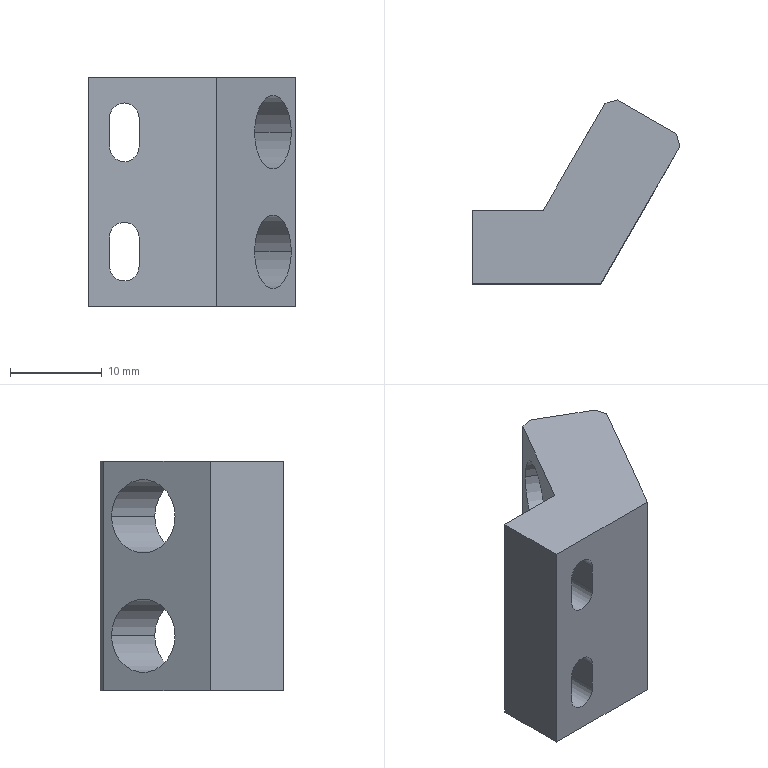Part | SolidWorks | features ICE 15, MoveFace 2, Chamfer 1, Extrusion 1 | 1 solid | 36 faces | box 22.618 x 20.004 x 25 mm | volume 4524 mm3 | plane 20 | cylinder 16 | commonest cylinder face diameters 3.2 x6 6 x6 8 x4
STEP:
#1=CARTESIAN_POINT('',(10.821,-32.,23.6));
#2=VERTEX_POINT('',#1);
#3=CARTESIAN_POINT('',(13.821,-32.,20.6));
#4=VERTEX_POINT('',#3);
#5=CARTESIAN_POINT('',(10.821,-32.,20.6));
#6=DIRECTION('',(0.,1.,0.));
#7=DIRECTION('',(0.,0.,1.));
#8=AXIS2_PLACEMENT_3D('',#5,#6,#7);
#9=CIRCLE('',#8,3.);
#10=EDGE_CURVE('',#2,#4,#9,.T.);
#11=ORIENTED_EDGE('',*,*,#10,.F.);
#12=CARTESIAN_POINT('',(10.821,-28.,23.6));
#13=VERTEX_POINT('',#12);
#14=CARTESIAN_POINT('',(10.821,-32.,23.6));
#15=DIRECTION('',(0.,1.,0.));
#16=VECTOR('',#15,1000.);
#17=LINE('',#14,#16);
#18=EDGE_CURVE('',#2,#13,#17,.T.);
#19=ORIENTED_EDGE('',*,*,#18,.T.);
#20=CARTESIAN_POINT('',(13.821,-28.,20.6));
#21=VERTEX_POINT('',#20);
#22=CARTESIAN_POINT('',(10.821,-28.,20.6));
#23=DIRECTION('',(0.,1.,0.));
#24=DIRECTION('',(0.,0.,1.));
#25=AXIS2_PLACEMENT_3D('',#22,#23,#24);
#26=CIRCLE('',#25,3.);
#27=EDGE_CURVE('',#13,#21,#26,.T.);
#28=ORIENTED_EDGE('',*,*,#27,.T.);
#29=CARTESIAN_POINT('',(13.821,-32.,20.6));
#30=DIRECTION('',(0.,1.,0.));
#31=VECTOR('',#30,1000.);
#32=LINE('',#29,#31);
#33=EDGE_CURVE('',#4,#21,#32,.T.);
#34=ORIENTED_EDGE('',*,*,#33,.F.);
#35=EDGE_LOOP('',(#11,#19,#28,#34));
#36=FACE_OUTER_BOUND('',#35,.T.);
#37=CARTESIAN_POINT('',(10.821,-32.,20.6));
#38=DIRECTION('',(0.,1.,0.));
#39=DIRECTION('',(0.,0.,1.));
#40=AXIS2_PLACEMENT_3D('',#37,#38,#39);
#41=CYLINDRICAL_SURFACE('',#40,3.);
#42=ADVANCED_FACE('',(#36),#41,.F.);
#43=CARTESIAN_POINT('',(10.821,-32.,10.6));
#44=VERTEX_POINT('',#43);
#45=CARTESIAN_POINT('',(13.821,-32.,7.6));
#46=VERTEX_POINT('',#45);
#47=CARTESIAN_POINT('',(10.821,-32.,7.6));
#48=DIRECTION('',(0.,1.,0.));
#49=DIRECTION('',(0.,0.,1.));
#50=AXIS2_PLACEMENT_3D('',#47,#48,#49);
#51=CIRCLE('',#50,3.);
#52=EDGE_CURVE('',#44,#46,#51,.T.);
#53=ORIENTED_EDGE('',*,*,#52,.F.);
#54=CARTESIAN_POINT('',(10.821,-28.,10.6));
#55=VERTEX_POINT('',#54);
#56=CARTESIAN_POINT('',(10.821,-32.,10.6));
#57=DIRECTION('',(0.,1.,0.));
#58=VECTOR('',#57,1000.);
#59=LINE('',#56,#58);
#60=EDGE_CURVE('',#44,#55,#59,.T.);
#61=ORIENTED_EDGE('',*,*,#60,.T.);
#62=CARTESIAN_POINT('',(13.821,-28.,7.6));
#63=VERTEX_POINT('',#62);
#64=CARTESIAN_POINT('',(10.821,-28.,7.6));
#65=DIRECTION('',(0.,1.,0.));
#66=DIRECTION('',(0.,0.,1.));
#67=AXIS2_PLACEMENT_3D('',#64,#65,#66);
#68=CIRCLE('',#67,3.);
#69=EDGE_CURVE('',#55,#63,#68,.T.);
#70=ORIENTED_EDGE('',*,*,#69,.T.);
#71=CARTESIAN_POINT('',(13.821,-32.,7.6));
#72=DIRECTION('',(0.,1.,0.));
#73=VECTOR('',#72,1000.);
#74=LINE('',#71,#73);
#75=EDGE_CURVE('',#46,#63,#74,.T.);
#76=ORIENTED_EDGE('',*,*,#75,.F.);
#77=EDGE_LOOP('',(#53,#61,#70,#76));
#78=FACE_OUTER_BOUND('',#77,.T.);
#79=CARTESIAN_POINT('',(10.821,-32.,7.6));
#80=DIRECTION('',(0.,1.,0.));
#81=DIRECTION('',(0.,0.,1.));
#82=AXIS2_PLACEMENT_3D('',#79,#80,#81);
#83=CYLINDRICAL_SURFACE('',#82,3.);
#84=ADVANCED_FACE('',(#78),#83,.F.);
#85=CARTESIAN_POINT('',(25.,-28.868,6.));
#86=VERTEX_POINT('',#85);
#87=CARTESIAN_POINT('',(29.,-21.939,6.));
#88=VERTEX_POINT('',#87);
#89=CARTESIAN_POINT('',(27.,-25.403,6.));
#90=DIRECTION('',(0.866,-0.5,0.));
#91=DIRECTION('',(-0.5,-0.866,0.));
#92=AXIS2_PLACEMENT_3D('',#89,#90,#91);
#93=CIRCLE('',#92,4.);
#94=EDGE_CURVE('',#86,#88,#93,.T.);
#95=ORIENTED_EDGE('',*,*,#94,.T.);
#96=CARTESIAN_POINT('',(20.84,-17.228,6.));
#97=VERTEX_POINT('',#96);
#98=CARTESIAN_POINT('',(52.301,-35.392,6.));
#99=DIRECTION('',(-0.866,0.5,0.));
#100=VECTOR('',#99,1000.);
#101=LINE('',#98,#100);
#102=EDGE_CURVE('',#88,#97,#101,.T.);
#103=ORIENTED_EDGE('',*,*,#102,.T.);
#104=CARTESIAN_POINT('',(16.84,-24.156,6.));
#105=VERTEX_POINT('',#104);
#106=CARTESIAN_POINT('',(18.84,-20.692,6.));
#107=DIRECTION('',(-0.866,0.5,0.));
#108=DIRECTION('',(0.5,0.866,0.));
#109=AXIS2_PLACEMENT_3D('',#106,#107,#108);
#110=CIRCLE('',#109,4.);
#111=EDGE_CURVE('',#97,#105,#110,.T.);
#112=ORIENTED_EDGE('',*,*,#111,.T.);
#113=CARTESIAN_POINT('',(48.301,-42.321,6.));
#114=DIRECTION('',(-0.866,0.5,0.));
#115=VECTOR('',#114,1000.);
#116=LINE('',#113,#115);
#117=EDGE_CURVE('',#86,#105,#116,.T.);
#118=ORIENTED_EDGE('',*,*,#117,.F.);
#119=EDGE_LOOP('',(#95,#103,#112,#118));
#120=FACE_OUTER_BOUND('',#119,.T.);
#121=CARTESIAN_POINT('',(50.301,-38.856,6.));
#122=DIRECTION('',(-0.866,0.5,0.));
#123=DIRECTION('',(-0.5,-0.866,0.));
#124=AXIS2_PLACEMENT_3D('',#121,#122,#123);
#125=CYLINDRICAL_SURFACE('',#124,4.);
#126=ADVANCED_FACE('',(#120),#125,.F.);
#127=CARTESIAN_POINT('',(25.,-28.868,19.));
#128=VERTEX_POINT('',#127);
#129=CARTESIAN_POINT('',(29.,-21.939,19.));
#130=VERTEX_POINT('',#129);
#131=CARTESIAN_POINT('',(27.,-25.403,19.));
#132=DIRECTION('',(0.866,-0.5,0.));
#133=DIRECTION('',(-0.5,-0.866,0.));
#134=AXIS2_PLACEMENT_3D('',#131,#132,#133);
#135=CIRCLE('',#134,4.);
#136=EDGE_CURVE('',#128,#130,#135,.T.);
#137=ORIENTED_EDGE('',*,*,#136,.T.);
#138=CARTESIAN_POINT('',(20.84,-17.228,19.));
#139=VERTEX_POINT('',#138);
#140=CARTESIAN_POINT('',(52.301,-35.392,19.));
#141=DIRECTION('',(-0.866,0.5,0.));
#142=VECTOR('',#141,1000.);
#143=LINE('',#140,#142);
#144=EDGE_CURVE('',#130,#139,#143,.T.);
#145=ORIENTED_EDGE('',*,*,#144,.T.);
#146=CARTESIAN_POINT('',(16.84,-24.156,19.));
#147=VERTEX_POINT('',#146);
#148=CARTESIAN_POINT('',(18.84,-20.692,19.));
#149=DIRECTION('',(-0.866,0.5,0.));
#150=DIRECTION('',(0.5,0.866,0.));
#151=AXIS2_PLACEMENT_3D('',#148,#149,#150);
#152=CIRCLE('',#151,4.);
#153=EDGE_CURVE('',#139,#147,#152,.T.);
#154=ORIENTED_EDGE('',*,*,#153,.T.);
#155=CARTESIAN_POINT('',(48.301,-42.321,19.));
#156=DIRECTION('',(-0.866,0.5,0.));
#157=VECTOR('',#156,1000.);
#158=LINE('',#155,#157);
#159=EDGE_CURVE('',#128,#147,#158,.T.);
#160=ORIENTED_EDGE('',*,*,#159,.F.);
#161=EDGE_LOOP('',(#137,#145,#154,#160));
#162=FACE_OUTER_BOUND('',#161,.T.);
#163=CARTESIAN_POINT('',(50.301,-38.856,19.));
#164=DIRECTION('',(-0.866,0.5,0.));
#165=DIRECTION('',(-0.5,-0.866,0.));
#166=AXIS2_PLACEMENT_3D('',#163,#164,#165);
#167=CYLINDRICAL_SURFACE('',#166,4.);
#168=ADVANCED_FACE('',(#162),#167,.F.);
#169=CARTESIAN_POINT('',(10.821,-36.,9.2));
#170=VERTEX_POINT('',#169);
#171=CARTESIAN_POINT('',(12.421,-36.,7.6));
#172=VERTEX_POINT('',#171);
#173=CARTESIAN_POINT('',(10.821,-36.,7.6));
#174=DIRECTION('',(0.,1.,0.));
#175=DIRECTION('',(0.,0.,1.));
#176=AXIS2_PLACEMENT_3D('',#173,#174,#175);
#177=CIRCLE('',#176,1.6);
#178=EDGE_CURVE('',#170,#172,#177,.T.);
#179=ORIENTED_EDGE('',*,*,#178,.F.);
#180=CARTESIAN_POINT('',(10.821,-32.,9.2));
#181=VERTEX_POINT('',#180);
#182=CARTESIAN_POINT('',(10.821,-38.,9.2));
#183=DIRECTION('',(0.,1.,0.));
#184=VECTOR('',#183,1000.);
#185=LINE('',#182,#184);
#186=EDGE_CURVE('',#170,#181,#185,.T.);
#187=ORIENTED_EDGE('',*,*,#186,.T.);
#188=CARTESIAN_POINT('',(12.421,-32.,7.6));
#189=VERTEX_POINT('',#188);
#190=CARTESIAN_POINT('',(10.821,-32.,7.6));
#191=DIRECTION('',(0.,-1.,0.));
#192=DIRECTION('',(0.,0.,1.));
#193=AXIS2_PLACEMENT_3D('',#190,#191,#192);
#194=CIRCLE('',#193,1.6);
#195=EDGE_CURVE('',#189,#181,#194,.T.);
#196=ORIENTED_EDGE('',*,*,#195,.F.);
#197=CARTESIAN_POINT('',(12.421,-38.,7.6));
#198=DIRECTION('',(0.,1.,0.));
#199=VECTOR('',#198,1000.);
#200=LINE('',#197,#199);
#201=EDGE_CURVE('',#172,#189,#200,.T.);
#202=ORIENTED_EDGE('',*,*,#201,.F.);
#203=EDGE_LOOP('',(#179,#187,#196,#202));
#204=FACE_OUTER_BOUND('',#203,.T.);
#205=CARTESIAN_POINT('',(10.821,-38.,7.6));
#206=DIRECTION('',(0.,1.,0.));
#207=DIRECTION('',(0.,0.,1.));
#208=AXIS2_PLACEMENT_3D('',#205,#206,#207);
#209=CYLINDRICAL_SURFACE('',#208,1.6);
#210=ADVANCED_FACE('',(#204),#209,.F.);
#211=CARTESIAN_POINT('',(10.821,-36.,22.2));
#212=VERTEX_POINT('',#211);
#213=CARTESIAN_POINT('',(12.421,-36.,20.6));
#214=VERTEX_POINT('',#213);
#215=CARTESIAN_POINT('',(10.821,-36.,20.6));
#216=DIRECTION('',(0.,1.,0.));
#217=DIRECTION('',(0.,0.,1.));
#218=AXIS2_PLACEMENT_3D('',#215,#216,#217);
#219=CIRCLE('',#218,1.6);
#220=EDGE_CURVE('',#212,#214,#219,.T.);
#221=ORIENTED_EDGE('',*,*,#220,.F.);
#222=CARTESIAN_POINT('',(10.821,-32.,22.2));
#223=VERTEX_POINT('',#222);
#224=CARTESIAN_POINT('',(10.821,-38.,22.2));
#225=DIRECTION('',(0.,1.,0.));
#226=VECTOR('',#225,1000.);
#227=LINE('',#224,#226);
#228=EDGE_CURVE('',#212,#223,#227,.T.);
#229=ORIENTED_EDGE('',*,*,#228,.T.);
#230=CARTESIAN_POINT('',(12.421,-32.,20.6));
#231=VERTEX_POINT('',#230);
#232=CARTESIAN_POINT('',(10.821,-32.,20.6));
#233=DIRECTION('',(0.,-1.,0.));
#234=DIRECTION('',(0.,0.,1.));
#235=AXIS2_PLACEMENT_3D('',#232,#233,#234);
#236=CIRCLE('',#235,1.6);
#237=EDGE_CURVE('',#231,#223,#236,.T.);
#238=ORIENTED_EDGE('',*,*,#237,.F.);
#239=CARTESIAN_POINT('',(12.421,-38.,20.6));
#240=DIRECTION('',(0.,1.,0.));
#241=VECTOR('',#240,1000.);
#242=LINE('',#239,#241);
#243=EDGE_CURVE('',#214,#231,#242,.T.);
#244=ORIENTED_EDGE('',*,*,#243,.F.);
#245=EDGE_LOOP('',(#221,#229,#238,#244));
#246=FACE_OUTER_BOUND('',#245,.T.);
#247=CARTESIAN_POINT('',(10.821,-38.,20.6));
#248=DIRECTION('',(0.,1.,0.));
#249=DIRECTION('',(0.,0.,1.));
#250=AXIS2_PLACEMENT_3D('',#247,#248,#249);
#251=CYLINDRICAL_SURFACE('',#250,1.6);
#252=ADVANCED_FACE('',(#246),#251,.F.);
#253=CARTESIAN_POINT('',(9.221,-32.,17.4));
#254=VERTEX_POINT('',#253);
#255=CARTESIAN_POINT('',(12.421,-32.,17.4));
#256=VERTEX_POINT('',#255);
#257=CARTESIAN_POINT('',(10.821,-32.,17.4));
#258=DIRECTION('',(0.,-1.,0.));
#259=DIRECTION('',(0.,0.,1.));
#260=AXIS2_PLACEMENT_3D('',#257,#258,#259);
#261=CIRCLE('',#260,1.6);
#262=EDGE_CURVE('',#254,#256,#261,.T.);
#263=ORIENTED_EDGE('',*,*,#262,.F.);
#264=CARTESIAN_POINT('',(9.221,-36.,17.4));
#265=VERTEX_POINT('',#264);
#266=CARTESIAN_POINT('',(9.221,-38.,17.4));
#267=DIRECTION('',(0.,1.,0.));
#268=VECTOR('',#267,1000.);
#269=LINE('',#266,#268);
#270=EDGE_CURVE('',#265,#254,#269,.T.);
#271=ORIENTED_EDGE('',*,*,#270,.F.);
#272=CARTESIAN_POINT('',(12.421,-36.,17.4));
#273=VERTEX_POINT('',#272);
#274=CARTESIAN_POINT('',(10.821,-36.,17.4));
#275=DIRECTION('',(0.,1.,0.));
#276=DIRECTION('',(0.,0.,1.));
#277=AXIS2_PLACEMENT_3D('',#274,#275,#276);
#278=CIRCLE('',#277,1.6);
#279=EDGE_CURVE('',#273,#265,#278,.T.);
#280=ORIENTED_EDGE('',*,*,#279,.F.);
#281=CARTESIAN_POINT('',(12.421,-38.,17.4));
#282=DIRECTION('',(0.,1.,0.));
#283=VECTOR('',#282,1000.);
#284=LINE('',#281,#283);
#285=EDGE_CURVE('',#273,#256,#284,.T.);
#286=ORIENTED_EDGE('',*,*,#285,.T.);
#287=EDGE_LOOP('',(#263,#271,#280,#286));
#288=FACE_OUTER_BOUND('',#287,.T.);
#289=CARTESIAN_POINT('',(10.821,-38.,17.4));
#290=DIRECTION('',(0.,1.,0.));
#291=DIRECTION('',(0.,0.,1.));
#292=AXIS2_PLACEMENT_3D('',#289,#290,#291);
#293=CYLINDRICAL_SURFACE('',#292,1.6);
#294=ADVANCED_FACE('',(#288),#293,.F.);
#295=ORIENTED_EDGE('',*,*,#228,.F.);
#296=CARTESIAN_POINT('',(9.221,-36.,20.6));
#297=VERTEX_POINT('',#296);
#298=CARTESIAN_POINT('',(10.821,-36.,20.6));
#299=DIRECTION('',(0.,1.,0.));
#300=DIRECTION('',(0.,0.,1.));
#301=AXIS2_PLACEMENT_3D('',#298,#299,#300);
#302=CIRCLE('',#301,1.6);
#303=EDGE_CURVE('',#297,#212,#302,.T.);
#304=ORIENTED_EDGE('',*,*,#303,.F.);
#305=CARTESIAN_POINT('',(9.221,-32.,20.6));
#306=VERTEX_POINT('',#305);
#307=CARTESIAN_POINT('',(9.221,-38.,20.6));
#308=DIRECTION('',(0.,1.,0.));
#309=VECTOR('',#308,1000.);
#310=LINE('',#307,#309);
#311=EDGE_CURVE('',#297,#306,#310,.T.);
#312=ORIENTED_EDGE('',*,*,#311,.T.);
#313=CARTESIAN_POINT('',(10.821,-32.,20.6));
#314=DIRECTION('',(0.,-1.,0.));
#315=DIRECTION('',(0.,0.,1.));
#316=AXIS2_PLACEMENT_3D('',#313,#314,#315);
#317=CIRCLE('',#316,1.6);
#318=EDGE_CURVE('',#223,#306,#317,.T.);
#319=ORIENTED_EDGE('',*,*,#318,.F.);
#320=EDGE_LOOP('',(#295,#304,#312,#319));
#321=FACE_OUTER_BOUND('',#320,.T.);
#322=CARTESIAN_POINT('',(10.821,-38.,20.6));
#323=DIRECTION('',(0.,1.,0.));
#324=DIRECTION('',(0.,0.,1.));
#325=AXIS2_PLACEMENT_3D('',#322,#323,#324);
#326=CYLINDRICAL_SURFACE('',#325,1.6);
#327=ADVANCED_FACE('',(#321),#326,.F.);
#328=CARTESIAN_POINT('',(12.421,-32.,17.4));
#329=DIRECTION('',(0.,0.,1.));
#330=VECTOR('',#329,1000.);
#331=LINE('',#328,#330);
#332=EDGE_CURVE('',#256,#231,#331,.T.);
#333=ORIENTED_EDGE('',*,*,#332,.F.);
#334=ORIENTED_EDGE('',*,*,#285,.F.);
#335=CARTESIAN_POINT('',(12.421,-36.,-6.));
#336=DIRECTION('',(0.,0.,-1.));
#337=VECTOR('',#336,1000.);
#338=LINE('',#335,#337);
#339=EDGE_CURVE('',#214,#273,#338,.T.);
#340=ORIENTED_EDGE('',*,*,#339,.F.);
#341=ORIENTED_EDGE('',*,*,#243,.T.);
#342=EDGE_LOOP('',(#333,#334,#340,#341));
#343=FACE_OUTER_BOUND('',#342,.T.);
#344=CARTESIAN_POINT('',(12.421,-38.,17.4));
#345=DIRECTION('',(1.,0.,0.));
#346=DIRECTION('',(0.,0.,-1.));
#347=AXIS2_PLACEMENT_3D('',#344,#345,#346);
#348=PLANE('',#347);
#349=ADVANCED_FACE('',(#343),#348,.F.);
#350=CARTESIAN_POINT('',(9.221,-32.,17.4));
#351=DIRECTION('',(0.,0.,-1.));
#352=VECTOR('',#351,1000.);
#353=LINE('',#350,#352);
#354=EDGE_CURVE('',#306,#254,#353,.T.);
#355=ORIENTED_EDGE('',*,*,#354,.F.);
#356=ORIENTED_EDGE('',*,*,#311,.F.);
#357=CARTESIAN_POINT('',(9.221,-36.,-6.));
#358=DIRECTION('',(0.,0.,1.));
#359=VECTOR('',#358,1000.);
#360=LINE('',#357,#359);
#361=EDGE_CURVE('',#265,#297,#360,.T.);
#362=ORIENTED_EDGE('',*,*,#361,.F.);
#363=ORIENTED_EDGE('',*,*,#270,.T.);
#364=EDGE_LOOP('',(#355,#356,#362,#363));
#365=FACE_OUTER_BOUND('',#364,.T.);
#366=CARTESIAN_POINT('',(9.221,-38.,17.4));
#367=DIRECTION('',(-1.,0.,0.));
#368=DIRECTION('',(0.,0.,1.));
#369=AXIS2_PLACEMENT_3D('',#366,#367,#368);
#370=PLANE('',#369);
#371=ADVANCED_FACE('',(#365),#370,.F.);
#372=CARTESIAN_POINT('',(9.221,-32.,4.4));
#373=VERTEX_POINT('',#372);
#374=CARTESIAN_POINT('',(12.421,-32.,4.4));
#375=VERTEX_POINT('',#374);
#376=CARTESIAN_POINT('',(10.821,-32.,4.4));
#377=DIRECTION('',(0.,-1.,0.));
#378=DIRECTION('',(0.,0.,1.));
#379=AXIS2_PLACEMENT_3D('',#376,#377,#378);
#380=CIRCLE('',#379,1.6);
#381=EDGE_CURVE('',#373,#375,#380,.T.);
#382=ORIENTED_EDGE('',*,*,#381,.F.);
#383=CARTESIAN_POINT('',(9.221,-36.,4.4));
#384=VERTEX_POINT('',#383);
#385=CARTESIAN_POINT('',(9.221,-38.,4.4));
#386=DIRECTION('',(0.,1.,0.));
#387=VECTOR('',#386,1000.);
#388=LINE('',#385,#387);
#389=EDGE_CURVE('',#384,#373,#388,.T.);
#390=ORIENTED_EDGE('',*,*,#389,.F.);
#391=CARTESIAN_POINT('',(12.421,-36.,4.4));
#392=VERTEX_POINT('',#391);
#393=CARTESIAN_POINT('',(10.821,-36.,4.4));
#394=DIRECTION('',(0.,1.,0.));
#395=DIRECTION('',(0.,0.,1.));
#396=AXIS2_PLACEMENT_3D('',#393,#394,#395);
#397=CIRCLE('',#396,1.6);
#398=EDGE_CURVE('',#392,#384,#397,.T.);
#399=ORIENTED_EDGE('',*,*,#398,.F.);
#400=CARTESIAN_POINT('',(12.421,-38.,4.4));
#401=DIRECTION('',(0.,1.,0.));
#402=VECTOR('',#401,1000.);
#403=LINE('',#400,#402);
#404=EDGE_CURVE('',#392,#375,#403,.T.);
#405=ORIENTED_EDGE('',*,*,#404,.T.);
#406=EDGE_LOOP('',(#382,#390,#399,#405));
#407=FACE_OUTER_BOUND('',#406,.T.);
#408=CARTESIAN_POINT('',(10.821,-38.,4.4));
#409=DIRECTION('',(0.,1.,0.));
#410=DIRECTION('',(0.,0.,1.));
#411=AXIS2_PLACEMENT_3D('',#408,#409,#410);
#412=CYLINDRICAL_SURFACE('',#411,1.6);
#413=ADVANCED_FACE('',(#407),#412,.F.);
#414=ORIENTED_EDGE('',*,*,#186,.F.);
#415=CARTESIAN_POINT('',(9.221,-36.,7.6));
#416=VERTEX_POINT('',#415);
#417=CARTESIAN_POINT('',(10.821,-36.,7.6));
#418=DIRECTION('',(0.,1.,0.));
#419=DIRECTION('',(0.,0.,1.));
#420=AXIS2_PLACEMENT_3D('',#417,#418,#419);
#421=CIRCLE('',#420,1.6);
#422=EDGE_CURVE('',#416,#170,#421,.T.);
#423=ORIENTED_EDGE('',*,*,#422,.F.);
#424=CARTESIAN_POINT('',(9.221,-32.,7.6));
#425=VERTEX_POINT('',#424);
#426=CARTESIAN_POINT('',(9.221,-38.,7.6));
#427=DIRECTION('',(0.,1.,0.));
#428=VECTOR('',#427,1000.);
#429=LINE('',#426,#428);
#430=EDGE_CURVE('',#416,#425,#429,.T.);
#431=ORIENTED_EDGE('',*,*,#430,.T.);
#432=CARTESIAN_POINT('',(10.821,-32.,7.6));
#433=DIRECTION('',(0.,-1.,0.));
#434=DIRECTION('',(0.,0.,1.));
#435=AXIS2_PLACEMENT_3D('',#432,#433,#434);
#436=CIRCLE('',#435,1.6);
#437=EDGE_CURVE('',#181,#425,#436,.T.);
#438=ORIENTED_EDGE('',*,*,#437,.F.);
#439=EDGE_LOOP('',(#414,#423,#431,#438));
#440=FACE_OUTER_BOUND('',#439,.T.);
#441=CARTESIAN_POINT('',(10.821,-38.,7.6));
#442=DIRECTION('',(0.,1.,0.));
#443=DIRECTION('',(0.,0.,1.));
#444=AXIS2_PLACEMENT_3D('',#441,#442,#443);
#445=CYLINDRICAL_SURFACE('',#444,1.6);
#446=ADVANCED_FACE('',(#440),#445,.F.);
#447=CARTESIAN_POINT('',(12.421,-32.,4.4));
#448=DIRECTION('',(0.,0.,1.));
#449=VECTOR('',#448,1000.);
#450=LINE('',#447,#449);
#451=EDGE_CURVE('',#375,#189,#450,.T.);
#452=ORIENTED_EDGE('',*,*,#451,.F.);
#453=ORIENTED_EDGE('',*,*,#404,.F.);
#454=CARTESIAN_POINT('',(12.421,-36.,-6.));
#455=DIRECTION('',(0.,0.,-1.));
#456=VECTOR('',#455,1000.);
#457=LINE('',#454,#456);
#458=EDGE_CURVE('',#172,#392,#457,.T.);
#459=ORIENTED_EDGE('',*,*,#458,.F.);
#460=ORIENTED_EDGE('',*,*,#201,.T.);
#461=EDGE_LOOP('',(#452,#453,#459,#460));
#462=FACE_OUTER_BOUND('',#461,.T.);
#463=CARTESIAN_POINT('',(12.421,-38.,4.4));
#464=DIRECTION('',(1.,0.,0.));
#465=DIRECTION('',(0.,0.,-1.));
#466=AXIS2_PLACEMENT_3D('',#463,#464,#465);
#467=PLANE('',#466);
#468=ADVANCED_FACE('',(#462),#467,.F.);
#469=CARTESIAN_POINT('',(9.221,-32.,4.4));
#470=DIRECTION('',(0.,0.,-1.));
#471=VECTOR('',#470,1000.);
#472=LINE('',#469,#471);
#473=EDGE_CURVE('',#425,#373,#472,.T.);
#474=ORIENTED_EDGE('',*,*,#473,.F.);
#475=ORIENTED_EDGE('',*,*,#430,.F.);
#476=CARTESIAN_POINT('',(9.221,-36.,-6.));
#477=DIRECTION('',(0.,0.,1.));
#478=VECTOR('',#477,1000.);
#479=LINE('',#476,#478);
#480=EDGE_CURVE('',#384,#416,#479,.T.);
#481=ORIENTED_EDGE('',*,*,#480,.F.);
#482=ORIENTED_EDGE('',*,*,#389,.T.);
#483=EDGE_LOOP('',(#474,#475,#481,#482));
#484=FACE_OUTER_BOUND('',#483,.T.);
#485=CARTESIAN_POINT('',(9.221,-38.,4.4));
#486=DIRECTION('',(-1.,0.,0.));
#487=DIRECTION('',(0.,0.,1.));
#488=AXIS2_PLACEMENT_3D('',#485,#486,#487);
#489=PLANE('',#488);
#490=ADVANCED_FACE('',(#484),#489,.F.);
#491=CARTESIAN_POINT('',(18.84,-20.692,19.));
#492=DIRECTION('',(-0.866,0.5,0.));
#493=DIRECTION('',(0.5,0.866,0.));
#494=AXIS2_PLACEMENT_3D('',#491,#492,#493);
#495=CIRCLE('',#494,4.);
#496=EDGE_CURVE('',#147,#139,#495,.T.);
#497=ORIENTED_EDGE('',*,*,#496,.F.);
#498=ORIENTED_EDGE('',*,*,#153,.F.);
#499=EDGE_LOOP('',(#497,#498));
#500=FACE_BOUND('',#499,.T.);
#501=CARTESIAN_POINT('',(18.84,-20.692,6.));
#502=DIRECTION('',(-0.866,0.5,0.));
#503=DIRECTION('',(0.5,0.866,0.));
#504=AXIS2_PLACEMENT_3D('',#501,#502,#503);
#505=CIRCLE('',#504,4.);
#506=EDGE_CURVE('',#105,#97,#505,.T.);
#507=ORIENTED_EDGE('',*,*,#506,.F.);
#508=ORIENTED_EDGE('',*,*,#111,.F.);
#509=EDGE_LOOP('',(#507,#508));
#510=FACE_BOUND('',#509,.T.);
#511=CARTESIAN_POINT('',(14.621,-28.,25.));
#512=VERTEX_POINT('',#511);
#513=CARTESIAN_POINT('',(14.621,-28.,0.));
#514=VERTEX_POINT('',#513);
#515=CARTESIAN_POINT('',(14.621,-28.,0.));
#516=DIRECTION('',(0.,0.,-1.));
#517=VECTOR('',#516,1000.);
#518=LINE('',#515,#517);
#519=EDGE_CURVE('',#512,#514,#518,.T.);
#520=ORIENTED_EDGE('',*,*,#519,.F.);
#521=CARTESIAN_POINT('',(21.34,-16.362,25.));
#522=VERTEX_POINT('',#521);
#523=CARTESIAN_POINT('',(21.84,-15.496,25.));
#524=DIRECTION('',(0.5,0.866,0.));
#525=VECTOR('',#524,1000.);
#526=LINE('',#523,#525);
#527=EDGE_CURVE('',#512,#522,#526,.T.);
#528=ORIENTED_EDGE('',*,*,#527,.T.);
#529=CARTESIAN_POINT('',(21.34,-16.362,0.));
#530=VERTEX_POINT('',#529);
#531=CARTESIAN_POINT('',(21.34,-16.362,0.));
#532=DIRECTION('',(0.,0.,-1.));
#533=VECTOR('',#532,1000.);
#534=LINE('',#531,#533);
#535=EDGE_CURVE('',#522,#530,#534,.T.);
#536=ORIENTED_EDGE('',*,*,#535,.T.);
#537=CARTESIAN_POINT('',(21.84,-15.496,0.));
#538=DIRECTION('',(0.5,0.866,0.));
#539=VECTOR('',#538,1000.);
#540=LINE('',#537,#539);
#541=EDGE_CURVE('',#514,#530,#540,.T.);
#542=ORIENTED_EDGE('',*,*,#541,.F.);
#543=EDGE_LOOP('',(#520,#528,#536,#542));
#544=FACE_OUTER_BOUND('',#543,.T.);
#545=CARTESIAN_POINT('',(21.84,-15.496,0.));
#546=DIRECTION('',(0.866,-0.5,0.));
#547=DIRECTION('',(0.5,0.866,0.));
#548=AXIS2_PLACEMENT_3D('',#545,#546,#547);
#549=PLANE('',#548);
#550=ADVANCED_FACE('',(#500,#510,#544),#549,.F.);
#551=CARTESIAN_POINT('',(29.134,-19.707,0.));
#552=VERTEX_POINT('',#551);
#553=CARTESIAN_POINT('',(22.706,-15.996,0.));
#554=VERTEX_POINT('',#553);
#555=CARTESIAN_POINT('',(53.301,-33.66,0.));
#556=DIRECTION('',(-0.866,0.5,0.));
#557=VECTOR('',#556,1000.);
#558=LINE('',#555,#557);
#559=EDGE_CURVE('',#552,#554,#558,.T.);
#560=ORIENTED_EDGE('',*,*,#559,.T.);
#561=CARTESIAN_POINT('',(22.706,-15.996,25.));
#562=VERTEX_POINT('',#561);
#563=CARTESIAN_POINT('',(22.706,-15.996,0.));
#564=DIRECTION('',(0.,0.,1.));
#565=VECTOR('',#564,1000.);
#566=LINE('',#563,#565);
#567=EDGE_CURVE('',#554,#562,#566,.T.);
#568=ORIENTED_EDGE('',*,*,#567,.T.);
#569=CARTESIAN_POINT('',(29.134,-19.707,25.));
#570=VERTEX_POINT('',#569);
#571=CARTESIAN_POINT('',(21.34,-15.207,25.));
#572=DIRECTION('',(0.866,-0.5,0.));
#573=VECTOR('',#572,1000.);
#574=LINE('',#571,#573);
#575=EDGE_CURVE('',#562,#570,#574,.T.);
#576=ORIENTED_EDGE('',*,*,#575,.T.);
#577=CARTESIAN_POINT('',(29.134,-19.707,0.));
#578=DIRECTION('',(0.,0.,-1.));
#579=VECTOR('',#578,1000.);
#580=LINE('',#577,#579);
#581=EDGE_CURVE('',#570,#552,#580,.T.);
#582=ORIENTED_EDGE('',*,*,#581,.T.);
#583=EDGE_LOOP('',(#560,#568,#576,#582));
#584=FACE_OUTER_BOUND('',#583,.T.);
#585=CARTESIAN_POINT('',(53.301,-33.66,0.));
#586=DIRECTION('',(-0.5,-0.866,0.));
#587=DIRECTION('',(0.866,-0.5,0.));
#588=AXIS2_PLACEMENT_3D('',#585,#586,#587);
#589=PLANE('',#588);
#590=ADVANCED_FACE('',(#584),#589,.F.);
#591=CARTESIAN_POINT('',(20.882,-36.,0.));
#592=VERTEX_POINT('',#591);
#593=CARTESIAN_POINT('',(6.882,-36.,0.));
#594=VERTEX_POINT('',#593);
#595=CARTESIAN_POINT('',(0.,-36.,0.));
#596=DIRECTION('',(-1.,0.,0.));
#597=VECTOR('',#596,1000.);
#598=LINE('',#595,#597);
#599=EDGE_CURVE('',#592,#594,#598,.T.);
#600=ORIENTED_EDGE('',*,*,#599,.T.);
#601=CARTESIAN_POINT('',(6.882,-28.,0.));
#602=VERTEX_POINT('',#601);
#603=CARTESIAN_POINT('',(6.882,-42.,0.));
#604=DIRECTION('',(0.,1.,0.));
#605=VECTOR('',#604,1000.);
#606=LINE('',#603,#605);
#607=EDGE_CURVE('',#594,#602,#606,.T.);
#608=ORIENTED_EDGE('',*,*,#607,.T.);
#609=CARTESIAN_POINT('',(20.882,-28.,0.));
#610=DIRECTION('',(1.,0.,0.));
#611=VECTOR('',#610,1000.);
#612=LINE('',#609,#611);
#613=EDGE_CURVE('',#602,#514,#612,.T.);
#614=ORIENTED_EDGE('',*,*,#613,.T.);
#615=ORIENTED_EDGE('',*,*,#541,.T.);
#616=CARTESIAN_POINT('',(22.706,-15.996,0.));
#617=DIRECTION('',(0.9659,0.2588,0.));
#618=VECTOR('',#617,1000.);
#619=LINE('',#616,#618);
#620=EDGE_CURVE('',#530,#554,#619,.T.);
#621=ORIENTED_EDGE('',*,*,#620,.T.);
#622=ORIENTED_EDGE('',*,*,#559,.F.);
#623=CARTESIAN_POINT('',(29.5,-21.073,0.));
#624=VERTEX_POINT('',#623);
#625=CARTESIAN_POINT('',(29.5,-21.073,0.));
#626=DIRECTION('',(0.2588,-0.9659,0.));
#627=VECTOR('',#626,1000.);
#628=LINE('',#625,#627);
#629=EDGE_CURVE('',#552,#624,#628,.T.);
#630=ORIENTED_EDGE('',*,*,#629,.T.);
#631=CARTESIAN_POINT('',(31.25,-18.042,0.));
#632=DIRECTION('',(-0.5,-0.866,0.));
#633=VECTOR('',#632,1000.);
#634=LINE('',#631,#633);
#635=EDGE_CURVE('',#624,#592,#634,.T.);
#636=ORIENTED_EDGE('',*,*,#635,.T.);
#637=EDGE_LOOP('',(#600,#608,#614,#615,#621,#622,#630,#636));
#638=FACE_OUTER_BOUND('',#637,.T.);
#639=CARTESIAN_POINT('',(0.,0.,0.));
#640=DIRECTION('',(0.,0.,1.));
#641=DIRECTION('',(1.,0.,0.));
#642=AXIS2_PLACEMENT_3D('',#639,#640,#641);
#643=PLANE('',#642);
#644=ADVANCED_FACE('',(#638),#643,.F.);
#645=ORIENTED_EDGE('',*,*,#136,.F.);
#646=CARTESIAN_POINT('',(27.,-25.403,19.));
#647=DIRECTION('',(0.866,-0.5,0.));
#648=DIRECTION('',(-0.5,-0.866,0.));
#649=AXIS2_PLACEMENT_3D('',#646,#647,#648);
#650=CIRCLE('',#649,4.);
#651=EDGE_CURVE('',#130,#128,#650,.T.);
#652=ORIENTED_EDGE('',*,*,#651,.F.);
#653=EDGE_LOOP('',(#645,#652));
#654=FACE_BOUND('',#653,.T.);
#655=ORIENTED_EDGE('',*,*,#94,.F.);
#656=CARTESIAN_POINT('',(27.,-25.403,6.));
#657=DIRECTION('',(0.866,-0.5,0.));
#658=DIRECTION('',(-0.5,-0.866,0.));
#659=AXIS2_PLACEMENT_3D('',#656,#657,#658);
#660=CIRCLE('',#659,4.);
#661=EDGE_CURVE('',#88,#86,#660,.T.);
#662=ORIENTED_EDGE('',*,*,#661,.F.);
#663=EDGE_LOOP('',(#655,#662));
#664=FACE_BOUND('',#663,.T.);
#665=ORIENTED_EDGE('',*,*,#635,.F.);
#666=CARTESIAN_POINT('',(29.5,-21.073,25.));
#667=VERTEX_POINT('',#666);
#668=CARTESIAN_POINT('',(29.5,-21.073,-18.));
#669=DIRECTION('',(0.,0.,1.));
#670=VECTOR('',#669,1000.);
#671=LINE('',#668,#670);
#672=EDGE_CURVE('',#624,#667,#671,.T.);
#673=ORIENTED_EDGE('',*,*,#672,.T.);
#674=CARTESIAN_POINT('',(20.882,-36.,25.));
#675=VERTEX_POINT('',#674);
#676=CARTESIAN_POINT('',(30.,-20.207,25.));
#677=DIRECTION('',(0.5,0.866,0.));
#678=VECTOR('',#677,1000.);
#679=LINE('',#676,#678);
#680=EDGE_CURVE('',#675,#667,#679,.T.);
#681=ORIENTED_EDGE('',*,*,#680,.F.);
#682=CARTESIAN_POINT('',(20.882,-36.,-18.));
#683=DIRECTION('',(0.,0.,1.));
#684=VECTOR('',#683,1000.);
#685=LINE('',#682,#684);
#686=EDGE_CURVE('',#592,#675,#685,.T.);
#687=ORIENTED_EDGE('',*,*,#686,.F.);
#688=EDGE_LOOP('',(#665,#673,#681,#687));
#689=FACE_OUTER_BOUND('',#688,.T.);
#690=CARTESIAN_POINT('',(30.,-20.207,-18.));
#691=DIRECTION('',(-0.866,0.5,0.));
#692=DIRECTION('',(-0.5,-0.866,0.));
#693=AXIS2_PLACEMENT_3D('',#690,#691,#692);
#694=PLANE('',#693);
#695=ADVANCED_FACE('',(#654,#664,#689),#694,.F.);
#696=ORIENTED_EDGE('',*,*,#144,.F.);
#697=ORIENTED_EDGE('',*,*,#651,.T.);
#698=ORIENTED_EDGE('',*,*,#159,.T.);
#699=ORIENTED_EDGE('',*,*,#496,.T.);
#700=EDGE_LOOP('',(#696,#697,#698,#699));
#701=FACE_OUTER_BOUND('',#700,.T.);
#702=CARTESIAN_POINT('',(50.301,-38.856,19.));
#703=DIRECTION('',(-0.866,0.5,0.));
#704=DIRECTION('',(-0.5,-0.866,0.));
#705=AXIS2_PLACEMENT_3D('',#702,#703,#704);
#706=CYLINDRICAL_SURFACE('',#705,4.);
#707=ADVANCED_FACE('',(#701),#706,.F.);
#708=ORIENTED_EDGE('',*,*,#102,.F.);
#709=ORIENTED_EDGE('',*,*,#661,.T.);
#710=ORIENTED_EDGE('',*,*,#117,.T.);
#711=ORIENTED_EDGE('',*,*,#506,.T.);
#712=EDGE_LOOP('',(#708,#709,#710,#711));
#713=FACE_OUTER_BOUND('',#712,.T.);
#714=CARTESIAN_POINT('',(50.301,-38.856,6.));
#715=DIRECTION('',(-0.866,0.5,0.));
#716=DIRECTION('',(-0.5,-0.866,0.));
#717=AXIS2_PLACEMENT_3D('',#714,#715,#716);
#718=CYLINDRICAL_SURFACE('',#717,4.);
#719=ADVANCED_FACE('',(#713),#718,.F.);
#720=CARTESIAN_POINT('',(6.882,-28.,25.));
#721=VERTEX_POINT('',#720);
#722=CARTESIAN_POINT('',(20.882,-28.,25.));
#723=DIRECTION('',(-1.,0.,0.));
#724=VECTOR('',#723,1000.);
#725=LINE('',#722,#724);
#726=EDGE_CURVE('',#512,#721,#725,.T.);
#727=ORIENTED_EDGE('',*,*,#726,.T.);
#728=CARTESIAN_POINT('',(6.882,-36.,25.));
#729=VERTEX_POINT('',#728);
#730=CARTESIAN_POINT('',(6.882,-42.,25.));
#731=DIRECTION('',(0.,1.,0.));
#732=VECTOR('',#731,1000.);
#733=LINE('',#730,#732);
#734=EDGE_CURVE('',#729,#721,#733,.T.);
#735=ORIENTED_EDGE('',*,*,#734,.F.);
#736=CARTESIAN_POINT('',(20.882,-36.,25.));
#737=DIRECTION('',(-1.,0.,0.));
#738=VECTOR('',#737,1000.);
#739=LINE('',#736,#738);
#740=EDGE_CURVE('',#675,#729,#739,.T.);
#741=ORIENTED_EDGE('',*,*,#740,.F.);
#742=ORIENTED_EDGE('',*,*,#680,.T.);
#743=CARTESIAN_POINT('',(29.5,-21.073,25.));
#744=DIRECTION('',(-0.2588,0.9659,0.));
#745=VECTOR('',#744,1000.);
#746=LINE('',#743,#745);
#747=EDGE_CURVE('',#667,#570,#746,.T.);
#748=ORIENTED_EDGE('',*,*,#747,.T.);
#749=ORIENTED_EDGE('',*,*,#575,.F.);
#750=CARTESIAN_POINT('',(22.706,-15.996,25.));
#751=DIRECTION('',(-0.9659,-0.2588,0.));
#752=VECTOR('',#751,1000.);
#753=LINE('',#750,#752);
#754=EDGE_CURVE('',#562,#522,#753,.T.);
#755=ORIENTED_EDGE('',*,*,#754,.T.);
#756=ORIENTED_EDGE('',*,*,#527,.F.);
#757=EDGE_LOOP('',(#727,#735,#741,#742,#748,#749,#755,#756));
#758=FACE_OUTER_BOUND('',#757,.T.);
#759=CARTESIAN_POINT('',(21.34,-15.207,25.));
#760=DIRECTION('',(0.,0.,-1.));
#761=DIRECTION('',(0.,1.,0.));
#762=AXIS2_PLACEMENT_3D('',#759,#760,#761);
#763=PLANE('',#762);
#764=ADVANCED_FACE('',(#758),#763,.F.);
#765=ORIENTED_EDGE('',*,*,#620,.F.);
#766=ORIENTED_EDGE('',*,*,#535,.F.);
#767=ORIENTED_EDGE('',*,*,#754,.F.);
#768=ORIENTED_EDGE('',*,*,#567,.F.);
#769=EDGE_LOOP('',(#765,#766,#767,#768));
#770=FACE_OUTER_BOUND('',#769,.T.);
#771=CARTESIAN_POINT('',(22.706,-15.996,0.));
#772=DIRECTION('',(0.2588,-0.9659,0.));
#773=DIRECTION('',(0.,0.,1.));
#774=AXIS2_PLACEMENT_3D('',#771,#772,#773);
#775=PLANE('',#774);
#776=ADVANCED_FACE('',(#770),#775,.F.);
#777=ORIENTED_EDGE('',*,*,#629,.F.);
#778=ORIENTED_EDGE('',*,*,#581,.F.);
#779=ORIENTED_EDGE('',*,*,#747,.F.);
#780=ORIENTED_EDGE('',*,*,#672,.F.);
#781=EDGE_LOOP('',(#777,#778,#779,#780));
#782=FACE_OUTER_BOUND('',#781,.T.);
#783=CARTESIAN_POINT('',(29.5,-21.073,-18.));
#784=DIRECTION('',(-0.9659,-0.2588,0.));
#785=DIRECTION('',(0.,0.,1.));
#786=AXIS2_PLACEMENT_3D('',#783,#784,#785);
#787=PLANE('',#786);
#788=ADVANCED_FACE('',(#782),#787,.F.);
#789=CARTESIAN_POINT('',(7.821,-28.,4.4));
#790=VERTEX_POINT('',#789);
#791=CARTESIAN_POINT('',(7.821,-28.,7.6));
#792=VERTEX_POINT('',#791);
#793=CARTESIAN_POINT('',(7.821,-28.,4.4));
#794=DIRECTION('',(0.,0.,1.));
#795=VECTOR('',#794,1000.);
#796=LINE('',#793,#795);
#797=EDGE_CURVE('',#790,#792,#796,.T.);
#798=ORIENTED_EDGE('',*,*,#797,.F.);
#799=CARTESIAN_POINT('',(13.821,-28.,4.4));
#800=VERTEX_POINT('',#799);
#801=CARTESIAN_POINT('',(10.821,-28.,4.4));
#802=DIRECTION('',(0.,1.,0.));
#803=DIRECTION('',(0.,0.,1.));
#804=AXIS2_PLACEMENT_3D('',#801,#802,#803);
#805=CIRCLE('',#804,3.);
#806=EDGE_CURVE('',#800,#790,#805,.T.);
#807=ORIENTED_EDGE('',*,*,#806,.F.);
#808=CARTESIAN_POINT('',(13.821,-28.,4.4));
#809=DIRECTION('',(0.,0.,-1.));
#810=VECTOR('',#809,1000.);
#811=LINE('',#808,#810);
#812=EDGE_CURVE('',#63,#800,#811,.T.);
#813=ORIENTED_EDGE('',*,*,#812,.F.);
#814=ORIENTED_EDGE('',*,*,#69,.F.);
#815=CARTESIAN_POINT('',(10.821,-28.,7.6));
#816=DIRECTION('',(0.,1.,0.));
#817=DIRECTION('',(0.,0.,1.));
#818=AXIS2_PLACEMENT_3D('',#815,#816,#817);
#819=CIRCLE('',#818,3.);
#820=EDGE_CURVE('',#792,#55,#819,.T.);
#821=ORIENTED_EDGE('',*,*,#820,.F.);
#822=EDGE_LOOP('',(#798,#807,#813,#814,#821));
#823=FACE_BOUND('',#822,.T.);
#824=CARTESIAN_POINT('',(7.821,-28.,17.4));
#825=VERTEX_POINT('',#824);
#826=CARTESIAN_POINT('',(7.821,-28.,20.6));
#827=VERTEX_POINT('',#826);
#828=CARTESIAN_POINT('',(7.821,-28.,17.4));
#829=DIRECTION('',(0.,0.,1.));
#830=VECTOR('',#829,1000.);
#831=LINE('',#828,#830);
#832=EDGE_CURVE('',#825,#827,#831,.T.);
#833=ORIENTED_EDGE('',*,*,#832,.F.);
#834=CARTESIAN_POINT('',(13.821,-28.,17.4));
#835=VERTEX_POINT('',#834);
#836=CARTESIAN_POINT('',(10.821,-28.,17.4));
#837=DIRECTION('',(0.,1.,0.));
#838=DIRECTION('',(0.,0.,1.));
#839=AXIS2_PLACEMENT_3D('',#836,#837,#838);
#840=CIRCLE('',#839,3.);
#841=EDGE_CURVE('',#835,#825,#840,.T.);
#842=ORIENTED_EDGE('',*,*,#841,.F.);
#843=CARTESIAN_POINT('',(13.821,-28.,17.4));
#844=DIRECTION('',(0.,0.,-1.));
#845=VECTOR('',#844,1000.);
#846=LINE('',#843,#845);
#847=EDGE_CURVE('',#21,#835,#846,.T.);
#848=ORIENTED_EDGE('',*,*,#847,.F.);
#849=ORIENTED_EDGE('',*,*,#27,.F.);
#850=CARTESIAN_POINT('',(10.821,-28.,20.6));
#851=DIRECTION('',(0.,1.,0.));
#852=DIRECTION('',(0.,0.,1.));
#853=AXIS2_PLACEMENT_3D('',#850,#851,#852);
#854=CIRCLE('',#853,3.);
#855=EDGE_CURVE('',#827,#13,#854,.T.);
#856=ORIENTED_EDGE('',*,*,#855,.F.);
#857=EDGE_LOOP('',(#833,#842,#848,#849,#856));
#858=FACE_BOUND('',#857,.T.);
#859=ORIENTED_EDGE('',*,*,#613,.F.);
#860=CARTESIAN_POINT('',(6.882,-28.,0.));
#861=DIRECTION('',(0.,0.,-1.));
#862=VECTOR('',#861,1000.);
#863=LINE('',#860,#862);
#864=EDGE_CURVE('',#721,#602,#863,.T.);
#865=ORIENTED_EDGE('',*,*,#864,.F.);
#866=ORIENTED_EDGE('',*,*,#726,.F.);
#867=ORIENTED_EDGE('',*,*,#519,.T.);
#868=EDGE_LOOP('',(#859,#865,#866,#867));
#869=FACE_OUTER_BOUND('',#868,.T.);
#870=CARTESIAN_POINT('',(0.,-28.,0.));
#871=DIRECTION('',(0.,-1.,0.));
#872=DIRECTION('',(0.,0.,-1.));
#873=AXIS2_PLACEMENT_3D('',#870,#871,#872);
#874=PLANE('',#873);
#875=ADVANCED_FACE('',(#823,#858,#869),#874,.F.);
#876=ORIENTED_EDGE('',*,*,#458,.T.);
#877=ORIENTED_EDGE('',*,*,#398,.T.);
#878=ORIENTED_EDGE('',*,*,#480,.T.);
#879=ORIENTED_EDGE('',*,*,#422,.T.);
#880=ORIENTED_EDGE('',*,*,#178,.T.);
#881=EDGE_LOOP('',(#876,#877,#878,#879,#880));
#882=FACE_BOUND('',#881,.T.);
#883=ORIENTED_EDGE('',*,*,#339,.T.);
#884=ORIENTED_EDGE('',*,*,#279,.T.);
#885=ORIENTED_EDGE('',*,*,#361,.T.);
#886=ORIENTED_EDGE('',*,*,#303,.T.);
#887=ORIENTED_EDGE('',*,*,#220,.T.);
#888=EDGE_LOOP('',(#883,#884,#885,#886,#887));
#889=FACE_BOUND('',#888,.T.);
#890=ORIENTED_EDGE('',*,*,#740,.T.);
#891=CARTESIAN_POINT('',(6.882,-36.,-6.));
#892=DIRECTION('',(0.,0.,-1.));
#893=VECTOR('',#892,1000.);
#894=LINE('',#891,#893);
#895=EDGE_CURVE('',#729,#594,#894,.T.);
#896=ORIENTED_EDGE('',*,*,#895,.T.);
#897=ORIENTED_EDGE('',*,*,#599,.F.);
#898=ORIENTED_EDGE('',*,*,#686,.T.);
#899=EDGE_LOOP('',(#890,#896,#897,#898));
#900=FACE_OUTER_BOUND('',#899,.T.);
#901=CARTESIAN_POINT('',(20.882,-36.,-6.));
#902=DIRECTION('',(0.,1.,0.));
#903=DIRECTION('',(0.,0.,1.));
#904=AXIS2_PLACEMENT_3D('',#901,#902,#903);
#905=PLANE('',#904);
#906=ADVANCED_FACE('',(#882,#889,#900),#905,.F.);
#907=ORIENTED_EDGE('',*,*,#734,.T.);
#908=ORIENTED_EDGE('',*,*,#864,.T.);
#909=ORIENTED_EDGE('',*,*,#607,.F.);
#910=ORIENTED_EDGE('',*,*,#895,.F.);
#911=EDGE_LOOP('',(#907,#908,#909,#910));
#912=FACE_OUTER_BOUND('',#911,.T.);
#913=CARTESIAN_POINT('',(6.882,-42.,0.));
#914=DIRECTION('',(1.,0.,0.));
#915=DIRECTION('',(0.,0.,-1.));
#916=AXIS2_PLACEMENT_3D('',#913,#914,#915);
#917=PLANE('',#916);
#918=ADVANCED_FACE('',(#912),#917,.F.);
#919=CARTESIAN_POINT('',(13.821,-32.,4.4));
#920=VERTEX_POINT('',#919);
#921=CARTESIAN_POINT('',(7.821,-32.,4.4));
#922=VERTEX_POINT('',#921);
#923=CARTESIAN_POINT('',(10.821,-32.,4.4));
#924=DIRECTION('',(0.,1.,0.));
#925=DIRECTION('',(0.,0.,1.));
#926=AXIS2_PLACEMENT_3D('',#923,#924,#925);
#927=CIRCLE('',#926,3.);
#928=EDGE_CURVE('',#920,#922,#927,.T.);
#929=ORIENTED_EDGE('',*,*,#928,.T.);
#930=CARTESIAN_POINT('',(7.821,-32.,7.6));
#931=VERTEX_POINT('',#930);
#932=CARTESIAN_POINT('',(7.821,-32.,4.4));
#933=DIRECTION('',(0.,0.,1.));
#934=VECTOR('',#933,1000.);
#935=LINE('',#932,#934);
#936=EDGE_CURVE('',#922,#931,#935,.T.);
#937=ORIENTED_EDGE('',*,*,#936,.T.);
#938=CARTESIAN_POINT('',(10.821,-32.,7.6));
#939=DIRECTION('',(0.,1.,0.));
#940=DIRECTION('',(0.,0.,1.));
#941=AXIS2_PLACEMENT_3D('',#938,#939,#940);
#942=CIRCLE('',#941,3.);
#943=EDGE_CURVE('',#931,#44,#942,.T.);
#944=ORIENTED_EDGE('',*,*,#943,.T.);
#945=ORIENTED_EDGE('',*,*,#52,.T.);
#946=CARTESIAN_POINT('',(13.821,-32.,4.4));
#947=DIRECTION('',(0.,0.,-1.));
#948=VECTOR('',#947,1000.);
#949=LINE('',#946,#948);
#950=EDGE_CURVE('',#46,#920,#949,.T.);
#951=ORIENTED_EDGE('',*,*,#950,.T.);
#952=EDGE_LOOP('',(#929,#937,#944,#945,#951));
#953=FACE_OUTER_BOUND('',#952,.T.);
#954=ORIENTED_EDGE('',*,*,#451,.T.);
#955=ORIENTED_EDGE('',*,*,#195,.T.);
#956=ORIENTED_EDGE('',*,*,#437,.T.);
#957=ORIENTED_EDGE('',*,*,#473,.T.);
#958=ORIENTED_EDGE('',*,*,#381,.T.);
#959=EDGE_LOOP('',(#954,#955,#956,#957,#958));
#960=FACE_BOUND('',#959,.T.);
#961=CARTESIAN_POINT('',(10.821,-32.,4.4));
#962=DIRECTION('',(0.,1.,0.));
#963=DIRECTION('',(0.,0.,1.));
#964=AXIS2_PLACEMENT_3D('',#961,#962,#963);
#965=PLANE('',#964);
#966=ADVANCED_FACE('',(#953,#960),#965,.T.);
#967=ORIENTED_EDGE('',*,*,#806,.T.);
#968=CARTESIAN_POINT('',(7.821,-32.,4.4));
#969=DIRECTION('',(0.,1.,0.));
#970=VECTOR('',#969,1000.);
#971=LINE('',#968,#970);
#972=EDGE_CURVE('',#922,#790,#971,.T.);
#973=ORIENTED_EDGE('',*,*,#972,.F.);
#974=ORIENTED_EDGE('',*,*,#928,.F.);
#975=CARTESIAN_POINT('',(13.821,-32.,4.4));
#976=DIRECTION('',(0.,1.,0.));
#977=VECTOR('',#976,1000.);
#978=LINE('',#975,#977);
#979=EDGE_CURVE('',#920,#800,#978,.T.);
#980=ORIENTED_EDGE('',*,*,#979,.T.);
#981=EDGE_LOOP('',(#967,#973,#974,#980));
#982=FACE_OUTER_BOUND('',#981,.T.);
#983=CARTESIAN_POINT('',(10.821,-32.,4.4));
#984=DIRECTION('',(0.,1.,0.));
#985=DIRECTION('',(0.,0.,1.));
#986=AXIS2_PLACEMENT_3D('',#983,#984,#985);
#987=CYLINDRICAL_SURFACE('',#986,3.);
#988=ADVANCED_FACE('',(#982),#987,.F.);
#989=ORIENTED_EDGE('',*,*,#812,.T.);
#990=ORIENTED_EDGE('',*,*,#979,.F.);
#991=ORIENTED_EDGE('',*,*,#950,.F.);
#992=ORIENTED_EDGE('',*,*,#75,.T.);
#993=EDGE_LOOP('',(#989,#990,#991,#992));
#994=FACE_OUTER_BOUND('',#993,.T.);
#995=CARTESIAN_POINT('',(13.821,-32.,4.4));
#996=DIRECTION('',(1.,0.,0.));
#997=DIRECTION('',(0.,0.,-1.));
#998=AXIS2_PLACEMENT_3D('',#995,#996,#997);
#999=PLANE('',#998);
#1000=ADVANCED_FACE('',(#994),#999,.F.);
#1001=ORIENTED_EDGE('',*,*,#60,.F.);
#1002=ORIENTED_EDGE('',*,*,#943,.F.);
#1003=CARTESIAN_POINT('',(7.821,-32.,7.6));
#1004=DIRECTION('',(0.,1.,0.));
#1005=VECTOR('',#1004,1000.);
#1006=LINE('',#1003,#1005);
#1007=EDGE_CURVE('',#931,#792,#1006,.T.);
#1008=ORIENTED_EDGE('',*,*,#1007,.T.);
#1009=ORIENTED_EDGE('',*,*,#820,.T.);
#1010=EDGE_LOOP('',(#1001,#1002,#1008,#1009));
#1011=FACE_OUTER_BOUND('',#1010,.T.);
#1012=CARTESIAN_POINT('',(10.821,-32.,7.6));
#1013=DIRECTION('',(0.,1.,0.));
#1014=DIRECTION('',(0.,0.,1.));
#1015=AXIS2_PLACEMENT_3D('',#1012,#1013,#1014);
#1016=CYLINDRICAL_SURFACE('',#1015,3.);
#1017=ADVANCED_FACE('',(#1011),#1016,.F.);
#1018=ORIENTED_EDGE('',*,*,#797,.T.);
#1019=ORIENTED_EDGE('',*,*,#1007,.F.);
#1020=ORIENTED_EDGE('',*,*,#936,.F.);
#1021=ORIENTED_EDGE('',*,*,#972,.T.);
#1022=EDGE_LOOP('',(#1018,#1019,#1020,#1021));
#1023=FACE_OUTER_BOUND('',#1022,.T.);
#1024=CARTESIAN_POINT('',(7.821,-32.,4.4));
#1025=DIRECTION('',(-1.,0.,0.));
#1026=DIRECTION('',(0.,0.,1.));
#1027=AXIS2_PLACEMENT_3D('',#1024,#1025,#1026);
#1028=PLANE('',#1027);
#1029=ADVANCED_FACE('',(#1023),#1028,.F.);
#1030=CARTESIAN_POINT('',(13.821,-32.,17.4));
#1031=VERTEX_POINT('',#1030);
#1032=CARTESIAN_POINT('',(7.821,-32.,17.4));
#1033=VERTEX_POINT('',#1032);
#1034=CARTESIAN_POINT('',(10.821,-32.,17.4));
#1035=DIRECTION('',(0.,1.,0.));
#1036=DIRECTION('',(0.,0.,1.));
#1037=AXIS2_PLACEMENT_3D('',#1034,#1035,#1036);
#1038=CIRCLE('',#1037,3.);
#1039=EDGE_CURVE('',#1031,#1033,#1038,.T.);
#1040=ORIENTED_EDGE('',*,*,#1039,.T.);
#1041=CARTESIAN_POINT('',(7.821,-32.,20.6));
#1042=VERTEX_POINT('',#1041);
#1043=CARTESIAN_POINT('',(7.821,-32.,17.4));
#1044=DIRECTION('',(0.,0.,1.));
#1045=VECTOR('',#1044,1000.);
#1046=LINE('',#1043,#1045);
#1047=EDGE_CURVE('',#1033,#1042,#1046,.T.);
#1048=ORIENTED_EDGE('',*,*,#1047,.T.);
#1049=CARTESIAN_POINT('',(10.821,-32.,20.6));
#1050=DIRECTION('',(0.,1.,0.));
#1051=DIRECTION('',(0.,0.,1.));
#1052=AXIS2_PLACEMENT_3D('',#1049,#1050,#1051);
#1053=CIRCLE('',#1052,3.);
#1054=EDGE_CURVE('',#1042,#2,#1053,.T.);
#1055=ORIENTED_EDGE('',*,*,#1054,.T.);
#1056=ORIENTED_EDGE('',*,*,#10,.T.);
#1057=CARTESIAN_POINT('',(13.821,-32.,17.4));
#1058=DIRECTION('',(0.,0.,-1.));
#1059=VECTOR('',#1058,1000.);
#1060=LINE('',#1057,#1059);
#1061=EDGE_CURVE('',#4,#1031,#1060,.T.);
#1062=ORIENTED_EDGE('',*,*,#1061,.T.);
#1063=EDGE_LOOP('',(#1040,#1048,#1055,#1056,#1062));
#1064=FACE_OUTER_BOUND('',#1063,.T.);
#1065=ORIENTED_EDGE('',*,*,#332,.T.);
#1066=ORIENTED_EDGE('',*,*,#237,.T.);
#1067=ORIENTED_EDGE('',*,*,#318,.T.);
#1068=ORIENTED_EDGE('',*,*,#354,.T.);
#1069=ORIENTED_EDGE('',*,*,#262,.T.);
#1070=EDGE_LOOP('',(#1065,#1066,#1067,#1068,#1069));
#1071=FACE_BOUND('',#1070,.T.);
#1072=CARTESIAN_POINT('',(10.821,-32.,17.4));
#1073=DIRECTION('',(0.,1.,0.));
#1074=DIRECTION('',(0.,0.,1.));
#1075=AXIS2_PLACEMENT_3D('',#1072,#1073,#1074);
#1076=PLANE('',#1075);
#1077=ADVANCED_FACE('',(#1064,#1071),#1076,.T.);
#1078=ORIENTED_EDGE('',*,*,#841,.T.);
#1079=CARTESIAN_POINT('',(7.821,-32.,17.4));
#1080=DIRECTION('',(0.,1.,0.));
#1081=VECTOR('',#1080,1000.);
#1082=LINE('',#1079,#1081);
#1083=EDGE_CURVE('',#1033,#825,#1082,.T.);
#1084=ORIENTED_EDGE('',*,*,#1083,.F.);
#1085=ORIENTED_EDGE('',*,*,#1039,.F.);
#1086=CARTESIAN_POINT('',(13.821,-32.,17.4));
#1087=DIRECTION('',(0.,1.,0.));
#1088=VECTOR('',#1087,1000.);
#1089=LINE('',#1086,#1088);
#1090=EDGE_CURVE('',#1031,#835,#1089,.T.);
#1091=ORIENTED_EDGE('',*,*,#1090,.T.);
#1092=EDGE_LOOP('',(#1078,#1084,#1085,#1091));
#1093=FACE_OUTER_BOUND('',#1092,.T.);
#1094=CARTESIAN_POINT('',(10.821,-32.,17.4));
#1095=DIRECTION('',(0.,1.,0.));
#1096=DIRECTION('',(0.,0.,1.));
#1097=AXIS2_PLACEMENT_3D('',#1094,#1095,#1096);
#1098=CYLINDRICAL_SURFACE('',#1097,3.);
#1099=ADVANCED_FACE('',(#1093),#1098,.F.);
#1100=ORIENTED_EDGE('',*,*,#847,.T.);
#1101=ORIENTED_EDGE('',*,*,#1090,.F.);
#1102=ORIENTED_EDGE('',*,*,#1061,.F.);
#1103=ORIENTED_EDGE('',*,*,#33,.T.);
#1104=EDGE_LOOP('',(#1100,#1101,#1102,#1103));
#1105=FACE_OUTER_BOUND('',#1104,.T.);
#1106=CARTESIAN_POINT('',(13.821,-32.,17.4));
#1107=DIRECTION('',(1.,0.,0.));
#1108=DIRECTION('',(0.,0.,-1.));
#1109=AXIS2_PLACEMENT_3D('',#1106,#1107,#1108);
#1110=PLANE('',#1109);
#1111=ADVANCED_FACE('',(#1105),#1110,.F.);
#1112=ORIENTED_EDGE('',*,*,#18,.F.);
#1113=ORIENTED_EDGE('',*,*,#1054,.F.);
#1114=CARTESIAN_POINT('',(7.821,-32.,20.6));
#1115=DIRECTION('',(0.,1.,0.));
#1116=VECTOR('',#1115,1000.);
#1117=LINE('',#1114,#1116);
#1118=EDGE_CURVE('',#1042,#827,#1117,.T.);
#1119=ORIENTED_EDGE('',*,*,#1118,.T.);
#1120=ORIENTED_EDGE('',*,*,#855,.T.);
#1121=EDGE_LOOP('',(#1112,#1113,#1119,#1120));
#1122=FACE_OUTER_BOUND('',#1121,.T.);
#1123=CARTESIAN_POINT('',(10.821,-32.,20.6));
#1124=DIRECTION('',(0.,1.,0.));
#1125=DIRECTION('',(0.,0.,1.));
#1126=AXIS2_PLACEMENT_3D('',#1123,#1124,#1125);
#1127=CYLINDRICAL_SURFACE('',#1126,3.);
#1128=ADVANCED_FACE('',(#1122),#1127,.F.);
#1129=ORIENTED_EDGE('',*,*,#832,.T.);
#1130=ORIENTED_EDGE('',*,*,#1118,.F.);
#1131=ORIENTED_EDGE('',*,*,#1047,.F.);
#1132=ORIENTED_EDGE('',*,*,#1083,.T.);
#1133=EDGE_LOOP('',(#1129,#1130,#1131,#1132));
#1134=FACE_OUTER_BOUND('',#1133,.T.);
#1135=CARTESIAN_POINT('',(7.821,-32.,17.4));
#1136=DIRECTION('',(-1.,0.,0.));
#1137=DIRECTION('',(0.,0.,1.));
#1138=AXIS2_PLACEMENT_3D('',#1135,#1136,#1137);
#1139=PLANE('',#1138);
#1140=ADVANCED_FACE('',(#1134),#1139,.F.);
#1141=CLOSED_SHELL('',(#42,#84,#126,#168,#210,#252,#294,#327,#349,#371,#413,#446,#468,#490,#550,#590,#644,#695,#707,#719,#764,#776,#788,#875,#906,#918,#966,#988,#1000,#1017,#1029,#1077,#1099,#1111,#1128,#1140));
#1142=MANIFOLD_SOLID_BREP('',#1141);
#1143=CARTESIAN_POINT('',(0.,0.,0.));
#1144=DIRECTION('',(0.,0.,1.));
#1145=DIRECTION('',(1.,0.,0.));
#1146=AXIS2_PLACEMENT_3D('',#1143,#1144,#1145);
#1147=(LENGTH_UNIT()NAMED_UNIT(*)SI_UNIT(.MILLI.,.METRE.));
#1148=UNCERTAINTY_MEASURE_WITH_UNIT(LENGTH_MEASURE(0.00001),#1147,'','');
#1149=(NAMED_UNIT(*)PLANE_ANGLE_UNIT()SI_UNIT($,.RADIAN.));
#1150=(NAMED_UNIT(*)SI_UNIT($,.STERADIAN.)SOLID_ANGLE_UNIT());
#1151=(GEOMETRIC_REPRESENTATION_CONTEXT(3)GLOBAL_UNCERTAINTY_ASSIGNED_CONTEXT((#1148))GLOBAL_UNIT_ASSIGNED_CONTEXT((#1147,#1149,#1150))REPRESENTATION_CONTEXT('',''));
#1152=ADVANCED_BREP_SHAPE_REPRESENTATION('',(#1142,#1146),#1151);